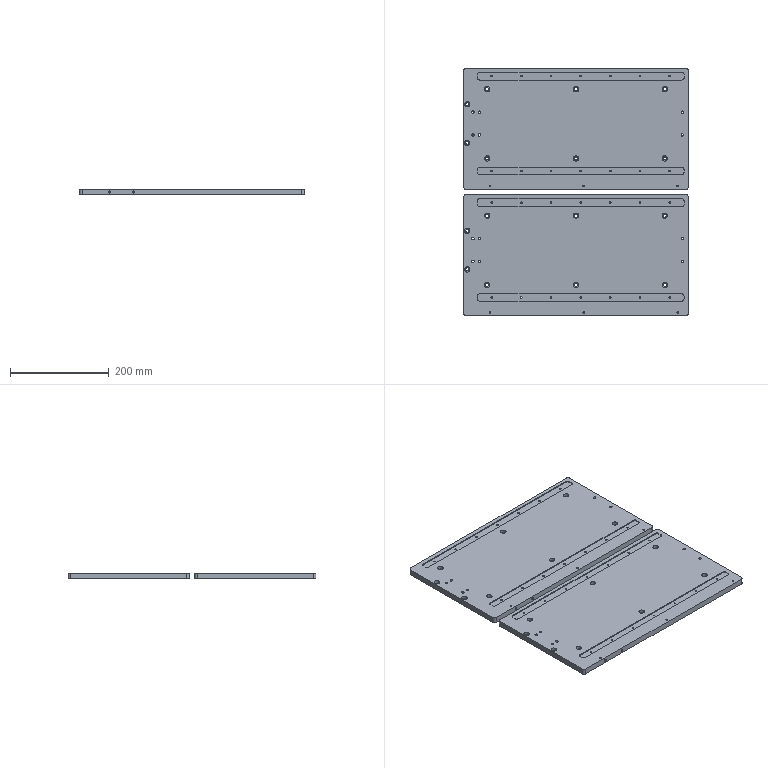Part | 2 solids | 158 faces | box 455 x 501 x 12 mm | volume 2604052 mm3 | cylinder 106 | plane 52 | commonest cylinder face diameters 3.2 x28 6.5 x16 11 x16 5 x12 10 x8 10.1 x8